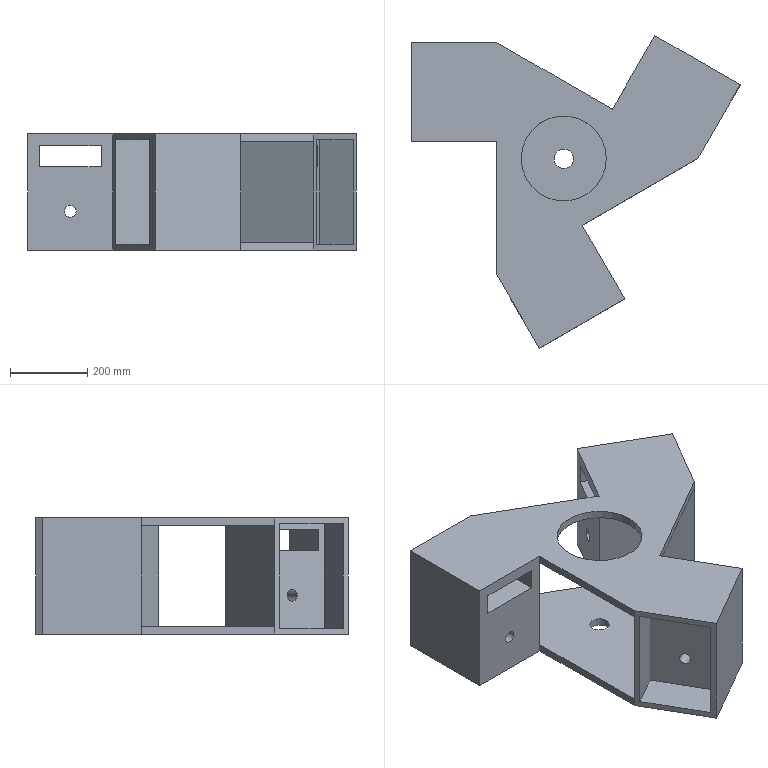Part | SolidWorks | features ICE 7, CirPattern 1, Extrusion 1 | 1 solid | 59 faces | box 849.615 x 808.551 x 300 mm | volume 36115158 mm3 | plane 49 | cylinder 10 | commonest cylinder face diameters 30 x6 50 x2 220 x2